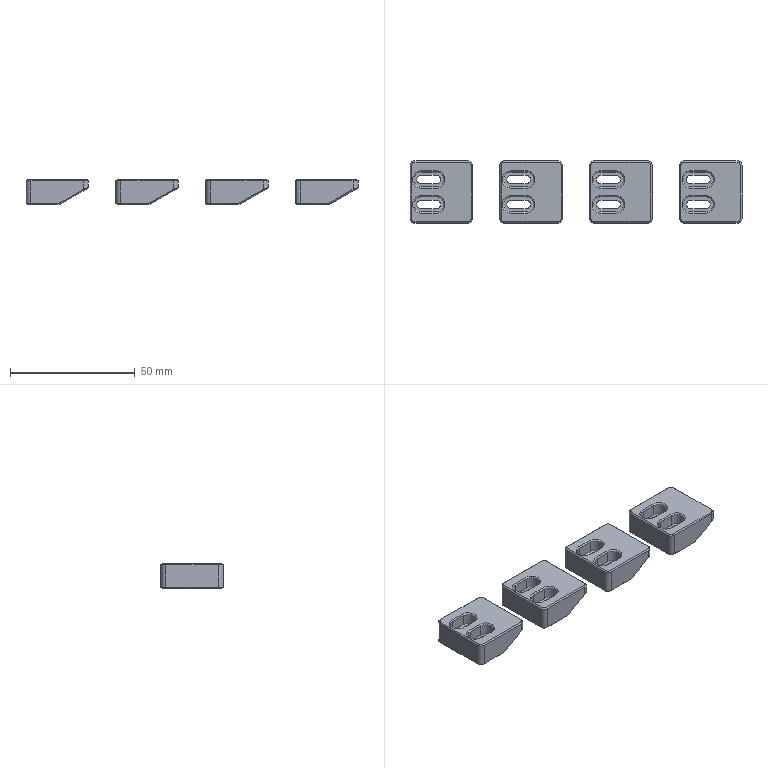NC program | NX | posted with a generic post | part box 133 x 25 x 10 mm
Lines 4147 to 5092 of 9691:
(ZLEVEL_PROFILE_1 , TOOL : D4R0.5)
N8274 T17 M6
N8276 G54
N8278 G17 G0 G90 X52.928 Y14.387 S9500 M3
N8280 G43 Z30. H17
N8282 Z1.492
N8284 G94 G1 Z-0.008 F1000.
N8286 X53.26 Y13.777
N8288 G3 X53.602 Y13.569 R0.4
N8290 G1 X54.449 Y13.548 F3500.
N8292 G2 X55.96 Y12.001 R1.548
N8294 G1 Y-12.002
N8296 G2 X54.447 Y-13.548 R1.546
N8298 G1 X53.731 Y-13.563
N8300 X53.733 Y-13.605 Z-0.012
N8302 Y-13.609 Z-0.017
N8304 X54.541 Y-13.585
N8306 G3 X56.077 Y-12.003 R1.583
N8308 G1 Y12.004
N8310 G3 X54.55 Y13.585 R1.583
N8312 G1 X53.602 Y13.618
N8314 Y13.651 Z-0.023
N8316 Y13.668 Z-0.03
N8318 G2 X54.868 Y13.578 R4.721
N8320 X56.185 Y12. R1.689
N8322 G1 Y-12.
N8324 G2 X54.868 Y-13.578 R1.689
N8326 X53.731 Y-13.668 R4.048
N8328 G1 Y-13.687 Z-0.037
N8330 Y-13.698 Z-0.045
N8332 G3 X54.868 Y-13.627 R4.522
N8334 X56.291 Y-12. R1.717
N8336 G1 Y12.
N8338 G3 X54.868 Y13.627 R1.717
N8340 X53.608 Y13.699 R5.373
N8342 G1 X53.616 Y13.731 Z-0.063
N8344 G2 X54.868 Y13.679 R7.793
N8346 X56.394 Y12. R1.79
N8348 G1 Y-12.
N8350 G2 X55.15 Y-13.595 R1.721
N8352 X53.731 Y-13.73 R4.1
N8354 G1 Y-13.759 Z-0.074
N8356 Y-13.768 Z-0.085
N8358 G3 X55.15 Y-13.649 R5.009
N8360 X56.495 Y-12. R1.779
N8362 G1 Y12.
N8364 G3 X55.077 Y13.665 R1.779
N8366 X53.626 Y13.768 R5.503
N8368 G1 X53.637 Y13.81 Z-0.108
N8370 G2 X55.15 Y13.693 R5.728
N8372 X56.594 Y12. R1.801
N8374 G1 Y-12.
N8376 G2 X55.431 Y-13.597 R1.737
N8378 X53.73 Y-13.81 R4.36
N8380 G1 X53.731 Y-13.827 Z-0.122
N8382 Y-13.84 Z-0.135
N8384 G3 X55.301 Y-13.696 R5.335
N8386 X56.693 Y-12. R1.829
N8388 G1 Y12.
N8390 G3 X55.301 Y13.696 R1.829
N8392 X53.731 Y13.84 R5.332
N8394 G1 X53.719 Y13.871 Z-0.164
N8396 G2 X55.311 Y13.739 R6.149
N8398 X56.79 Y12. R1.88
N8400 G1 Y-12.
N8402 G2 X55.311 Y-13.739 R1.88
N8404 X53.719 Y-13.871 R6.154
N8406 G1 X53.731 Y-13.904 Z-0.196
N8408 X54.565 Y-13.888
N8410 G3 X55.925 Y-13.542 R3.077
N8412 X56.886 Y-12. R1.785
N8414 G1 Y12.
N8416 G3 X55.431 Y13.747 R1.879
N8418 X53.731 Y13.904 R6.066
N8420 G1 X53.733 Y13.938 Z-0.231
N8422 G2 X55.431 Y13.785 R6.166
N8424 X56.835 Y12.686 R2.074
N8426 G1 X56.968 Y12.122
N8428 X56.981 Y12.
N8430 Y-12.
N8432 G2 X55.58 Y-13.743 R1.894
N8434 X53.733 Y-13.938 R5.951
N8436 G1 X53.724 Y-13.976 Z-0.269
N8438 X54.467 Y-13.962
N8440 G3 X55.991 Y-13.621 R3.913
N8442 X57.075 Y-12. R1.833
N8444 G1 Y12.002
N8446 G3 X56.499 Y13.277 R1.7
N8448 X55.431 Y13.824 R2.438
N8450 X53.724 Y13.976 R6.331
N8452 G1 X53.729 Y14.016 Z-0.309
N8454 G2 X55.994 Y13.678 R5.445
N8456 X57.168 Y12. R1.869
N8458 G1 Y-12.
N8460 G2 X55.994 Y-13.678 R1.869
N8462 X53.729 Y-14.016 R5.443
N8464 G1 X53.724 Y-14.058 Z-0.351
N8466 G3 X55.994 Y-13.721 R5.597
N8468 X57.259 Y-12. R1.893
N8470 G1 Y12.
N8472 G3 X55.994 Y13.721 R1.893
N8474 X53.724 Y14.058 R5.598
N8476 G1 X53.461 Y14.104 Z-0.397
N8478 X54.232 Y14.102
N8480 G2 X56.262 Y13.652 R4.836
N8482 X57.349 Y12. R1.88
N8484 G1 Y-12.
N8486 G2 X56.262 Y-13.652 R1.88
N8488 X54.232 Y-14.102 R4.837
N8490 G1 X53.461 Y-14.104
N8492 Y-14.151 Z-0.444
N8494 X54.2
N8496 G3 X56.513 Y-13.569 R4.883
N8498 G1 X56.557 Y-13.545
N8500 G3 X57.437 Y-12. R1.869
N8502 G1 Y12.005
N8504 G3 X56.504 Y13.572 R1.783
N8506 G1 X56.276 Y13.697
N8508 G3 X54.188 Y14.15 R5.072
N8510 G1 X53.461 Y14.151
N8512 Y14.2 Z-0.493
N8514 X54.196 Y14.199
N8516 G2 X56.554 Y13.598 R4.96
N8518 X57.522 Y12. R1.853
N8520 G1 Y-12.
N8522 G2 X56.517 Y-13.624 R1.88
N8524 X54.183 Y-14.2 R5.017
N8526 G1 X53.461
N8528 X53.742 Y-14.249 Z-0.542
N8530 G3 X56.557 Y-13.655 R5.49
N8532 X57.608 Y-12. R1.902
N8534 G1 Y12.
N8536 G3 X56.557 Y13.648 R1.875
N8538 X53.742 Y14.249 R5.381
N8540 G1 Y14.299 Z-0.592
N8542 G2 X56.808 Y13.557 R5.411
N8544 X57.694 Y12.005 R1.802
N8546 G1 Y-12.005
N8548 G2 X56.809 Y-13.557 R1.802
N8550 X53.742 Y-14.299 R5.409
N8552 G1 Y-14.324 Z-0.617
N8554 Y-14.349 Z-0.642
N8556 G3 X56.551 Y-13.749 R5.466
N8558 G1 X56.658 Y-13.695
N8560 G3 X57.78 Y-12. R1.933
N8562 G1 Y12.
N8564 G3 X56.658 Y13.695 R1.933
N8566 G1 X56.551 Y13.749
N8568 G3 X53.742 Y14.349 R5.467
N8570 G1 X53.747 Y14.374 Z-0.667
N8572 X53.751 Y14.399 Z-0.692
N8574 G2 X56.522 Y13.807 R5.412
N8576 G1 X56.745 Y13.695
N8578 G2 X57.867 Y12. R1.933
N8580 G1 Y-12.
N8582 G2 X56.745 Y-13.695 R1.933
N8584 G1 X56.522 Y-13.807
N8586 G2 X53.751 Y-14.399 R5.411
N8588 G1 X53.752 Y-14.424 Z-0.717
N8590 X53.753 Y-14.449 Z-0.742
N8592 G3 X56.493 Y-13.864 R5.353
N8594 G1 X56.832 Y-13.695
N8596 G3 X57.954 Y-12. R1.933
N8598 G1 Y12.
N8600 G3 X56.832 Y13.695 R1.933
N8602 G1 X56.493 Y13.864
N8604 G3 X53.753 Y14.449 R5.354
N8606 G1 X53.755 Y14.474 Z-0.767
N8608 X53.756 Y14.499 Z-0.792
N8610 G2 X56.465 Y13.922 R5.316
N8612 G1 X56.918 Y13.695
N8614 G2 X58.04 Y12. R1.933
N8616 G1 Y-12.
N8618 G2 X56.918 Y-13.695 R1.936
N8620 G1 X56.465 Y-13.922
N8622 G2 X53.756 Y-14.499 R5.315
N8624 G1 X53.758 Y-14.524 Z-0.817
N8626 X53.759 Y-14.549 Z-0.842
N8628 G3 X56.436 Y-13.98 R5.379
N8630 G1 X57.005 Y-13.695
N8632 G3 X58.127 Y-12. R1.933
N8634 G1 Y12.
N8636 G3 X57.005 Y13.695 R1.933
N8638 G1 X56.436 Y13.98
N8640 G3 X53.759 Y14.549 R5.266
N8642 G1 X53.76 Y14.574 Z-0.867
N8644 X53.762 Y14.599 Z-0.892
N8646 G2 X56.407 Y14.037 R5.221
N8648 G1 X57.091 Y13.695
N8650 G2 X58.214 Y12. R1.933
N8652 G1 Y-12.
N8654 G2 X57.091 Y-13.695 R1.933
N8656 G1 X56.407 Y-14.037
N8658 G2 X53.762 Y-14.599 R5.191
N8660 G1 X53.763 Y-14.624 Z-0.917
N8662 X53.764 Y-14.649 Z-0.942
N8664 G3 X56.378 Y-14.095 R5.178
N8666 G1 X57.178 Y-13.695
N8668 G3 X58.3 Y-12. R1.933
N8670 G1 Y12.
N8672 G3 X57.178 Y13.695 R1.933
N8674 G1 X56.378 Y14.095
N8676 G3 X53.764 Y14.649 R5.179
N8678 G1 X53.891 Y14.666 Z-0.959
N8680 X54.018 Y14.682 Z-0.976
N8682 X54.145 Y14.696 Z-0.992
N8684 G2 X56.349 Y14.153 R5.038
N8686 G1 X57.265 Y13.695
N8688 G2 X58.387 Y12. R1.933
N8690 G1 Y-12.
N8692 G2 X57.265 Y-13.695 R1.936
N8694 G1 X56.349 Y-14.153
N8696 G2 X54.135 Y-14.695 R5.021
N8698 G1 X54.275 Y-14.707 Z-1.005
N8700 X54.414 Y-14.711 Z-1.017
N8702 X54.553 Y-14.714 Z-1.03
N8704 X54.692 Y-14.71 Z-1.042
N8706 G3 X56.351 Y-14.195 R5.063
N8708 G1 X57.351 Y-13.695
N8710 G3 X58.473 Y-12. R1.933
N8712 G1 Y12.
N8714 G3 X57.351 Y13.695 R1.933
N8716 G1 X56.351 Y14.195
N8718 G3 X54.692 Y14.71 R5.042
N8720 G1 X54.825 Y14.714 Z-1.059
N8722 X54.957 Y14.705 Z-1.076
N8724 X55.087 Y14.694 Z-1.092
N8726 G2 X56.438 Y14.195 R5.676
N8728 G1 X57.438 Y13.695
N8730 G2 X58.56 Y12. R1.933
N8732 G1 Y-12.
N8734 G2 X57.438 Y-13.695 R1.933
N8736 G1 X56.438 Y-14.195
N8738 G2 X55.089 Y-14.694 R5.697
N8740 G1 X55.228 Y-14.691 Z-1.117
N8742 X55.363 Y-14.671 Z-1.142
N8744 G3 X56.353 Y-14.281 R6.036
N8746 G1 X57.524 Y-13.695
N8748 G3 X58.647 Y-12. R1.942
N8750 G1 Y12.
N8752 G3 X57.524 Y13.695 R1.933
N8754 G1 X56.355 Y14.28
N8756 G3 X55.361 Y14.671 R6.026
N8758 G1 X55.476 Y14.662 Z-1.167
N8760 X55.59 Y14.648 Z-1.192
N8762 G2 X56.405 Y14.298 R7.558
N8764 G1 X57.611 Y13.695
N8766 G2 X58.733 Y12. R1.933
N8768 G1 Y-12.
N8770 G2 X57.611 Y-13.695 R1.933
N8772 G1 X56.396 Y-14.303
N8774 G2 X55.593 Y-14.647 R7.478
N8776 G1 X55.688 Y-14.64 Z-1.217
N8778 X55.779 Y-14.624 Z-1.242
N8780 G3 X56.473 Y-14.308 R10.854
N8782 G1 X57.698 Y-13.695
N8784 G3 X58.82 Y-12. R1.933
N8786 G1 Y12.
N8788 G3 X57.698 Y13.695 R1.933
N8790 G1 X56.698 Y14.195
N8792 G3 X55.777 Y14.625 R16.455
N8794 G1 X55.852 Y14.617 Z-1.267
N8796 X55.926 Y14.606 Z-1.292
N8798 X56.784 Y14.195
N8800 X57.784 Y13.695
N8802 G2 X58.906 Y12. R1.933
N8804 G1 Y-12.
N8806 G2 X57.784 Y-13.695 R1.942
N8808 G1 X56.784 Y-14.195
N8810 X55.929 Y-14.606
N8812 X56.057 Y-14.593 Z-1.342
N8814 X56.871 Y-14.195
N8816 X57.871 Y-13.695
N8818 G3 X58.993 Y-12. R1.933
N8820 G1 Y12.
N8822 G3 X57.871 Y13.695 R1.933
N8824 G1 X56.871 Y14.195
N8826 X56.055 Y14.592
N8828 X56.168 Y14.582 Z-1.392
N8830 X56.276 Y14.533
N8832 X56.957 Y14.195
N8834 X57.957 Y13.695
N8836 G2 X59.08 Y12. R1.933
N8838 G1 Y-12.
N8840 G2 X57.957 Y-13.695 R1.933
N8842 G1 X56.957 Y-14.195
N8844 X56.276 Y-14.534
N8846 X56.17 Y-14.583
N8848 X56.281 Y-14.575 Z-1.442
N8850 X57.044 Y-14.195
N8852 X58.044 Y-13.695
N8854 G3 X59.166 Y-12. R1.936
N8856 G1 Y12.
N8858 G3 X58.044 Y13.695 R1.933
N8860 G1 X57.044 Y14.195
N8862 X56.279 Y14.574
N8864 X56.367 Y14.571 Z-1.492
N8866 X57.131 Y14.195
N8868 X58.131 Y13.695
N8870 G2 X59.253 Y12. R1.933
N8872 G1 Y-12.
N8874 G2 X58.131 Y-13.695 R1.933
N8876 G1 X57.131 Y-14.195
N8878 X56.369 Y-14.571
N8880 X56.457 Z-1.542
N8882 X56.557 Y-14.524
N8884 X57.217 Y-14.195
N8886 X58.217 Y-13.695
N8888 G3 X59.339 Y-12. R1.933
N8890 G1 Y12.
N8892 G3 X58.217 Y13.695 R1.933
N8894 G1 X57.217 Y14.195
N8896 X56.557 Y14.523
N8898 X56.455 Y14.57
N8900 X56.545 Y14.571 Z-1.592
N8902 X57.304 Y14.195
N8904 X58.304 Y13.695
N8906 G2 X59.426 Y12. R1.933
N8908 G1 Y-12.
N8910 G2 X58.304 Y-13.695 R1.933
N8912 G1 X57.304 Y-14.195
N8914 X56.547 Y-14.572
N8916 X56.634 Y-14.569 Z-1.642
N8918 X57.39 Y-14.195
N8920 X58.39 Y-13.695
N8922 G3 X59.513 Y-12. R1.936
N8924 G1 Y12.
N8926 G3 X58.39 Y13.695 R1.933
N8928 G1 X57.39 Y14.195
N8930 X56.633 Y14.569
N8932 X56.721 Y14.567 Z-1.692
N8934 X56.838 Y14.512
N8936 X57.477 Y14.195
N8938 X58.477 Y13.695
N8940 G2 X59.599 Y12. R1.933
N8942 G1 Y-12.
N8944 G2 X58.477 Y-13.695 R1.933
N8946 G1 X57.477 Y-14.195
N8948 X56.838 Y-14.513
N8950 X56.722 Y-14.568
N8952 X56.812 Y-14.569 Z-1.742
N8954 X56.838 Y-14.557
N8956 X57.564 Y-14.195
N8958 X58.564 Y-13.695
N8960 G3 X59.686 Y-12. R1.933
N8962 G1 Y12.
N8964 G3 X58.564 Y13.695 R1.933
N8966 G1 X57.564 Y14.195
N8968 X56.838 Y14.556
N8970 X56.81 Y14.568
N8972 X56.898 Y14.567 Z-1.792
N8974 X57.65 Y14.195
N8976 X58.65 Y13.695
N8978 G2 X59.772 Y12. R1.933
N8980 G1 Y-12.
N8982 G2 X58.65 Y-13.695 R1.942
N8984 G1 X57.65 Y-14.195
N8986 X56.899 Y-14.567
N8988 X56.987 Y-14.565 Z-1.842
N8990 X57.12 Y-14.503
N8992 X57.737 Y-14.195
N8994 X58.737 Y-13.695
N8996 G3 X59.859 Y-12. R1.933
N8998 G1 Y12.
N9000 G3 X58.737 Y13.695 R1.933
N9002 G1 X57.737 Y14.195
N9004 X57.12 Y14.502
N9006 X56.986 Y14.565
N9008 X57.075 Y14.566 Z-1.892
N9010 X57.12 Y14.546
N9012 X57.823 Y14.195
N9014 X58.824 Y13.695
N9016 G2 X59.946 Y12. R1.933
N9018 G1 Y-12.
N9020 G2 X58.824 Y-13.695 R1.933
N9022 G1 X57.823 Y-14.195
N9024 X57.12 Y-14.546
N9026 X57.077 Y-14.566
N9028 X57.165 Y-14.565 Z-1.942
N9030 X57.91 Y-14.195
N9032 X58.91 Y-13.695
N9034 G3 X60.032 Y-12. R1.942
N9036 G1 Y12.
N9038 G3 X58.91 Y13.695 R1.933
N9040 G1 X57.91 Y14.195
N9042 X57.164 Y14.565
N9044 X57.252 Y14.563 Z-1.992
N9046 X57.401 Y14.492
N9048 X57.997 Y14.195
N9050 X58.997 Y13.695
N9052 G2 X60.119 Y12. R1.933
N9054 G1 Y-12.
N9056 G2 X58.997 Y-13.695 R1.933
N9058 G1 X57.997 Y-14.195
N9060 X57.401 Y-14.493
N9062 X57.253 Y-14.563
N9064 X57.342 Z-2.042
N9066 X57.401 Y-14.536
N9068 X58.083 Y-14.195
N9070 X59.083 Y-13.695
N9072 G3 X60.205 Y-12. R1.933
N9074 G1 Y12.
N9076 G3 X59.083 Y13.695 R1.933
N9078 G1 X58.083 Y14.195
N9080 X57.401 Y14.535
N9082 X57.341 Y14.563
N9084 X57.43 Z-2.092
N9086 X58.17 Y14.195
N9088 X59.17 Y13.695
N9090 G2 X60.292 Y12. R1.933
N9092 G1 Y-12.
N9094 G2 X59.17 Y-13.695 R1.936
N9096 G1 X58.17 Y-14.195
N9098 X57.43 Y-14.563
N9100 X57.518 Y-14.561 Z-2.142
N9102 X58.256 Y-14.195
N9104 X59.257 Y-13.695
N9106 G3 X60.379 Y-12. R1.933
N9108 G1 Y12.
N9110 G3 X59.257 Y13.695 R1.933
N9112 G1 X58.256 Y14.195
N9114 X57.517 Y14.561
N9116 X57.606 Y14.56 Z-2.192
N9118 X57.683 Y14.525
N9120 X58.343 Y14.195
N9122 X59.343 Y13.695
N9124 G2 X60.465 Y12. R1.933
N9126 G1 Y-12.
N9128 G2 X59.343 Y-13.695 R1.933
N9130 G1 X58.343 Y-14.195
N9132 X57.683 Y-14.526
N9134 X57.607 Y-14.561
N9136 X57.696 Y-14.562 Z-2.242
N9138 X58.43 Y-14.195
N9140 X59.43 Y-13.695
N9142 G3 X60.552 Y-12. R1.933
N9144 G1 Y12.
N9146 G3 X59.43 Y13.695 R1.933
N9148 G1 X58.43 Y14.195
N9150 X57.695 Y14.562
N9152 X57.782 Y14.559 Z-2.292
N9154 X58.516 Y14.195
N9156 X59.516 Y13.695
N9158 G2 X60.638 Y12. R1.933
N9160 G1 Y-12.
N9162 G2 X59.516 Y-13.695 R1.936
N9164 G1 X58.516 Y-14.195
N9166 X57.782 Y-14.559
N9168 X57.87 Y-14.558 Z-2.342
N9170 X57.964 Y-14.515
N9172 X58.603 Y-14.195
N9174 X59.603 Y-13.695
N9176 G3 X60.725 Y-12. R1.933
N9178 G1 Y12.
N9180 G3 X59.603 Y13.695 R1.933
N9182 G1 X58.603 Y14.195
N9184 X57.964 Y14.514
N9186 X57.869 Y14.558
N9188 X57.958 Y14.56 Z-2.392
N9190 X58.689 Y14.195
N9192 X59.69 Y13.695
N9194 G2 X60.812 Y12. R1.933
N9196 G1 Y-12.
N9198 G2 X59.69 Y-13.695 R1.933
N9200 G1 X58.689 Y-14.195
N9202 X57.959 Y-14.561
N9204 X58.045 Y-14.558 Z-2.442
N9206 X58.776 Y-14.195
N9208 X59.776 Y-13.695
N9210 G3 X60.898 Y-12. R1.942
N9212 G1 Y12.
N9214 G3 X59.776 Y13.695 R1.933
N9216 G1 X58.776 Y14.195
N9218 X58.045 Y14.557
N9220 X58.132 Y14.556 Z-2.492
N9222 X58.246 Y14.504
N9224 X58.863 Y14.195
N9226 X59.863 Y13.695
N9228 G2 X60.985 Y12. R1.933
N9230 G1 Y-12.
N9232 G2 X59.863 Y-13.695 R1.933
N9234 G1 X58.863 Y-14.195
N9236 X58.246 Y-14.504
N9238 X58.133 Y-14.557
N9240 X58.221 Y-14.558 Z-2.542
N9242 X58.246 Y-14.547
N9244 X58.949 Y-14.195
N9246 X59.949 Y-13.695
N9248 G3 X61.071 Y-12. R1.933
N9250 G1 Y12.
N9252 G3 X59.949 Y13.695 R1.933
N9254 G1 X58.949 Y14.195
N9256 X58.246 Y14.547
N9258 X58.221 Y14.558
N9260 X58.308 Y14.556 Z-2.592
N9262 X59.036 Y14.195
N9264 X60.036 Y13.695
N9266 G2 X61.158 Y12. R1.933
N9268 G1 Y-12.
N9270 G2 X60.036 Y-13.695 R1.942
N9272 G1 X59.036 Y-14.195
N9274 X58.308 Y-14.556
N9276 X58.395 Y-14.555 Z-2.642
N9278 X58.527 Y-14.493
N9280 X59.122 Y-14.195
N9282 X60.123 Y-13.695
N9284 G3 X61.245 Y-12. R1.933
N9286 G1 Y12.
N9288 G3 X60.123 Y13.695 R1.933
N9290 G1 X59.122 Y14.195
N9292 X58.527 Y14.493
N9294 X58.395 Y14.555
N9296 X58.483 Y14.556 Z-2.692
N9298 X58.527 Y14.536
N9300 X59.209 Y14.195
N9302 X60.209 Y13.695
N9304 G2 X61.331 Y12. R1.933
N9306 G1 Y-12.
N9308 G2 X60.209 Y-13.695 R1.933
N9310 G1 X59.209 Y-14.195
N9312 X58.527 Y-14.536
N9314 X58.484 Y-14.556
N9316 X58.571 Y-14.555 Z-2.742
N9318 X59.296 Y-14.195
N9320 X60.296 Y-13.695
N9322 G3 X61.418 Y-12. R1.936
N9324 G1 Y12.
N9326 G3 X60.296 Y13.695 R1.933
N9328 G1 X59.296 Y14.195
N9330 X58.571 Y14.555
N9332 X58.658 Y14.553 Z-2.792
N9334 X59.382 Y14.195
N9336 X60.382 Y13.695
N9338 G2 X61.504 Y12. R1.933
N9340 G1 Y-12.
N9342 G2 X60.382 Y-13.695 R1.933
N9344 G1 X59.382 Y-14.195
N9346 X58.658 Y-14.553
N9348 X58.746 Y-14.554 Z-2.842
N9350 X58.809 Y-14.526
N9352 X59.469 Y-14.195
N9354 X60.469 Y-13.695
N9356 G3 X61.591 Y-12. R1.933
N9358 G1 Y12.
N9360 G3 X60.469 Y13.695 R1.933
N9362 G1 X59.469 Y14.195
N9364 X58.809 Y14.525
N9366 X58.746 Y14.554
N9368 X58.834 Z-2.892
N9370 X59.556 Y14.195
N9372 X60.556 Y13.695
N9374 G2 X61.678 Y12. R1.933
N9376 G1 Y-12.
N9378 G2 X60.556 Y-13.695 R1.933
N9380 G1 X59.556 Y-14.195
N9382 X58.835 Y-14.555
N9384 X58.921 Y-14.552 Z-2.942
N9386 X59.642 Y-14.195
N9388 X60.642 Y-13.695
N9390 G3 X61.764 Y-12. R1.936
N9392 G1 Y12.
N9394 G3 X60.642 Y13.695 R1.933
N9396 G1 X59.642 Y14.195
N9398 X58.921 Y14.552
N9400 X59.009 Z-2.992
N9402 X59.09 Y14.514
N9404 X59.729 Y14.195
N9406 X60.729 Y13.695
N9408 G2 X61.851 Y12. R1.933
N9410 G1 Y-12.
N9412 G2 X60.729 Y-13.695 R1.933
N9414 G1 X59.729 Y-14.195
N9416 X59.09 Y-14.515
N9418 X59.009 Y-14.552
N9420 X59.098 Y-14.554 Z-3.042
N9422 X59.815 Y-14.195
N9424 X60.815 Y-13.695
N9426 G3 X61.937 Y-12. R1.933
N9428 G1 Y12.
N9430 G3 X60.815 Y13.695 R1.933
N9432 G1 X59.815 Y14.195
N9434 X59.097 Y14.554
N9436 X59.183 Y14.551 Z-3.092
N9438 X59.902 Y14.195
N9440 X60.902 Y13.695
N9442 G2 X62.024 Y12. R1.933
N9444 G1 Y-12.
N9446 G2 X60.902 Y-13.695 R1.942
N9448 G1 X59.902 Y-14.195
N9450 X59.184 Y-14.551
N9452 X59.271 Y-14.55 Z-3.142
N9454 X59.372 Y-14.504
N9456 X59.989 Y-14.195
N9458 X60.989 Y-13.695
N9460 G3 X62.111 Y-12. R1.933
N9462 G1 Y12.
N9464 G3 X60.989 Y13.695 R1.933
N9466 G1 X59.989 Y14.195
N9468 X59.372 Y14.504
N9470 X59.271 Y14.55
N9472 X59.359 Y14.552 Z-3.192
N9474 X60.075 Y14.195
N9476 X61.075 Y13.695
N9478 G2 X62.197 Y12. R1.933
N9480 G1 Y-12.
N9482 G2 X61.075 Y-13.695 R1.933
N9484 G1 X60.075 Y-14.195
N9486 X59.36 Y-14.553
N9488 X59.446 Y-14.55 Z-3.242
N9490 X60.162 Y-14.195
N9492 X61.162 Y-13.695
N9494 G3 X62.284 Y-12. R1.942
N9496 G1 Y12.
N9498 G3 X61.162 Y13.695 R1.933
N9500 G1 X60.162 Y14.195
N9502 X59.445 Y14.55
N9504 X59.532 Y14.549 Z-3.292
N9506 X59.653 Y14.493
N9508 X60.248 Y14.195
N9510 X61.248 Y13.695
N9512 G2 X62.37 Y12. R1.933
N9514 G1 Y-12.
N9516 G2 X61.248 Y-13.695 R1.933
N9518 G1 X60.248 Y-14.195
N9520 X59.653 Y-14.493
N9522 X59.533 Y-14.549
N9524 X59.621 Y-14.551 Z-3.342
N9526 X59.653 Y-14.536
N9528 X60.335 Y-14.195
N9530 X61.335 Y-13.695
N9532 G3 X62.457 Y-12. R1.933
N9534 G1 Y12.
N9536 G3 X61.335 Y13.695 R1.933
N9538 G1 X60.335 Y14.195
N9540 X59.653 Y14.536
N9542 X59.62 Y14.551
N9544 X59.707 Y14.55 Z-3.392
N9546 X60.422 Y14.195
N9548 X61.422 Y13.695
N9550 G2 X62.544 Y12. R1.933
N9552 G1 Y-12.
N9554 G2 X61.422 Y-13.695 R1.936
N9556 G1 X60.422 Y-14.195
N9558 X59.707 Y-14.55
N9560 X59.794 Y-14.548 Z-3.442
N9562 X59.935 Y-14.482
N9564 X60.508 Y-14.195
N9566 X61.508 Y-13.695
N9568 G3 X62.63 Y-12. R1.933
N9570 G1 Y12.
N9572 G3 X61.508 Y13.695 R1.933
N9574 G1 X60.508 Y14.195
N9576 X59.935 Y14.482
N9578 X59.793 Y14.548
N9580 X59.881 Y14.549 Z-3.492
N9582 X59.935 Y14.525
N9584 X60.595 Y14.195
N9586 X61.595 Y13.695
N9588 G2 X62.717 Y12. R1.933
N9590 G1 Y-12.
N9592 G2 X61.595 Y-13.695 R1.933
N9594 G1 X60.595 Y-14.195
N9596 X59.935 Y-14.526
N9598 X59.882 Y-14.549
N9600 X59.969 Z-3.542
N9602 X60.681 Y-14.195
N9604 X61.681 Y-13.695
N9606 G3 X62.803 Y-12. R1.933
N9608 G1 Y12.
N9610 G3 X61.681 Y13.695 R1.933
N9612 G1 X60.681 Y14.195
N9614 X59.969 Y14.55
N9616 X60.055 Y14.547 Z-3.592
N9618 X60.768 Y14.195
N9620 X61.768 Y13.695
N9622 G2 X62.89 Y12. R1.933
N9624 G1 Y-12.
N9626 G2 X61.768 Y-13.695 R1.936
N9628 G1 X60.768 Y-14.195
N9630 X60.056 Y-14.547
N9632 X60.143 Y-14.548 Z-3.642
N9634 X60.216 Y-14.515
N9636 X60.855 Y-14.195
N9638 X61.855 Y-13.695
N9640 G3 X62.977 Y-12. R1.933
N9642 G1 Y12.
N9644 G3 X61.855 Y13.695 R1.933
N9646 G1 X60.855 Y14.195
N9648 X60.216 Y14.514
N9650 X60.143 Y14.548
N9652 X60.231 Y14.549 Z-3.692
N9654 X60.941 Y14.195
N9656 X61.941 Y13.695
N9658 G2 X63.063 Y12. R1.933
N9660 G1 Y-12.
N9662 G2 X61.941 Y-13.695 R1.933
N9664 G1 X60.941 Y-14.195
N9666 X60.231 Y-14.549
N9668 X60.317 Y-14.546 Z-3.742
N9670 X61.028 Y-14.195
N9672 X62.028 Y-13.695
N9674 G3 X63.15 Y-12. R1.942
N9676 G1 Y12.
N9678 G3 X62.028 Y13.695 R1.933
N9680 G1 X61.028 Y14.195
N9682 X60.317 Y14.546
N9684 X60.404 Z-3.792
N9686 X60.497 Y14.504
N9688 X61.114 Y14.195
N9690 X62.114 Y13.695
N9692 G2 X63.236 Y12. R1.933
N9694 G1 Y-12.
N9696 G2 X62.114 Y-13.695 R1.933
N9698 G1 X61.114 Y-14.195
N9700 X60.497 Y-14.504
N9702 X60.405 Y-14.546
N9704 X60.493 Y-14.549 Z-3.842
N9706 X61.201 Y-14.195
N9708 X62.201 Y-13.695
N9710 G3 X63.323 Y-12. R1.933
N9712 G1 Y12.
N9714 G3 X62.201 Y13.695 R1.933
N9716 G1 X61.201 Y14.195
N9718 X60.492 Y14.549
N9720 X60.578 Y14.546 Z-3.892
N9722 X61.288 Y14.195
N9724 X62.288 Y13.695
N9726 G2 X63.41 Y12. R1.933
N9728 G1 Y-12.
N9730 G2 X62.288 Y-13.695 R1.942
N9732 G1 X61.288 Y-14.195
N9734 X60.579 Y-14.546
N9736 X60.666 Y-14.545 Z-3.942
N9738 X60.779 Y-14.493
N9740 X61.374 Y-14.195
N9742 X62.374 Y-13.695
N9744 G3 X63.496 Y-12. R1.933
N9746 G1 Y12.
N9748 G3 X62.374 Y13.695 R1.933
N9750 G1 X61.374 Y14.195
N9752 X60.779 Y14.493
N9754 X60.665 Y14.545
N9756 X60.753 Y14.547 Z-3.992
N9758 X60.779 Y14.536
N9760 X61.461 Y14.195
N9762 X62.461 Y13.695
N9764 G2 X63.583 Y12. R1.933
N9766 G1 Y-12.
N9768 G2 X62.461 Y-13.695 R1.933
N9770 G1 X61.461 Y-14.195
N9772 X60.779 Y-14.536
N9774 X60.754 Y-14.547
N9776 X60.841 Y-14.545 Z-4.042
N9778 X61.547 Y-14.195
N9780 X62.547 Y-13.695
N9782 G3 X63.669 Y-12. R1.936
N9784 G1 Y12.
N9786 G3 X62.547 Y13.695 R1.933
N9788 G1 X61.547 Y14.195
N9790 X60.84 Y14.546
N9792 X60.927 Y14.544 Z-4.092
N9794 X61.06 Y14.482
N9796 X61.634 Y14.195
N9798 X62.634 Y13.695
N9800 G2 X63.756 Y12. R1.933
N9802 G1 Y-12.
N9804 G2 X62.634 Y-13.695 R1.933
N9806 G1 X61.634 Y-14.195
N9808 X61.06 Y-14.482
N9810 X60.928 Y-14.544
N9812 X61.016 Y-14.545 Z-4.142
N9814 X61.06 Y-14.526
N9816 X61.721 Y-14.195
N9818 X62.721 Y-13.695
N9820 G3 X63.843 Y-12. R1.933
N9822 G1 Y12.
N9824 G3 X62.721 Y13.695 R1.933
N9826 G1 X61.721 Y14.195
N9828 X61.06 Y14.525
N9830 X61.015 Y14.546
N9832 X61.102 Y14.545 Z-4.192
N9834 X61.807 Y14.195
N9836 X62.807 Y13.695
N9838 G2 X63.929 Y12. R1.933
N9840 G1 Y-12.
N9842 G2 X62.807 Y-13.695 R1.933
N9844 G1 X61.807 Y-14.195
N9846 X61.103 Y-14.545
N9848 X61.189 Y-14.543 Z-4.242
N9850 X61.894 Y-14.195
N9852 X62.894 Y-13.695
N9854 G3 X64.016 Y-12. R1.936
N9856 G1 Y12.
N9858 G3 X62.894 Y13.695 R1.933
N9860 G1 X61.894 Y14.195
N9862 X61.188 Y14.543
N9864 X61.276 Y14.544 Z-4.292
N9866 X61.342 Y14.514
N9868 X61.98 Y14.195
N9870 X62.98 Y13.695
N9872 G2 X64.102 Y12. R1.933
N9874 G1 Y-12.
N9876 G2 X62.98 Y-13.695 R1.933
N9878 G1 X61.98 Y-14.195
N9880 X61.342 Y-14.515
N9882 X61.277 Y-14.544
N9884 X61.365 Y-14.545 Z-4.342
N9886 X62.067 Y-14.195
N9888 X63.067 Y-13.695
N9890 G3 X64.189 Y-12. R1.933
N9892 G1 Y12.
N9894 G3 X63.067 Y13.695 R1.933
N9896 G1 X62.067 Y14.195
N9898 X61.364 Y14.545
N9900 X61.45 Y14.543 Z-4.392
N9902 X62.154 Y14.195
N9904 X63.154 Y13.695
N9906 G2 X64.276 Y12. R1.933
N9908 G1 Y-12.
N9910 G2 X63.154 Y-13.695 R1.942
N9912 G1 X62.154 Y-14.195
N9914 X61.451 Y-14.542
N9916 X61.538 Z-4.442
N9918 X61.623 Y-14.504
N9920 X62.24 Y-14.195
N9922 X63.24 Y-13.695
N9924 G3 X64.362 Y-12. R1.933
N9926 G1 Y12.
N9928 G3 X63.24 Y13.695 R1.933
N9930 G1 X62.24 Y14.195
N9932 X61.623 Y14.504
N9934 X61.537 Y14.543
N9936 X61.626 Y14.546 Z-4.492
N9938 X62.327 Y14.195
N9940 X63.327 Y13.695
N9942 G2 X64.449 Y12. R1.933
N9944 G1 Y-12.
N9946 G2 X63.327 Y-13.695 R1.933
N9948 G1 X62.327 Y-14.195
N9950 X61.627 Y-14.545
N9952 X61.713 Y-14.542 Z-4.542
N9954 X62.413 Y-14.195
N9956 X63.413 Y-13.695
N9958 G3 X64.535 Y-12. R1.942
N9960 G1 Y12.
N9962 G3 X63.413 Y13.695 R1.933
N9964 G1 X62.413 Y14.195
N9966 X61.711 Y14.542
N9968 X61.799 Y14.541 Z-4.592
N9970 X61.905 Y14.493
N9972 X62.5 Y14.195
N9974 X63.5 Y13.695
N9976 G2 X64.622 Y12. R1.933
N9978 G1 Y-12.
N9980 G2 X63.5 Y-13.695 R1.933
N9982 G1 X62.5 Y-14.195
N9984 X61.905 Y-14.493
N9986 X61.8 Y-14.541
N9988 X61.889 Y-14.543 Z-4.642
N9990 X62.587 Y-14.195
N9992 X63.587 Y-13.695
N9994 G3 X64.709 Y-12. R1.933
N9996 G1 Y12.
N9998 G3 X63.587 Y13.695 R1.933
N10000 G1 X62.587 Y14.195
N10002 X61.887 Y14.544
N10004 X61.973 Y14.542 Z-4.692
N10006 X62.673 Y14.195
N10008 X63.673 Y13.695
N10010 G2 X64.795 Y12. R1.933
N10012 G1 Y-12.
N10014 G2 X63.673 Y-13.695 R1.936
N10016 G1 X62.673 Y-14.195
N10018 X61.975 Y-14.541
N10020 X62.061 Y-14.54 Z-4.742
N10022 X62.186 Y-14.482
N10024 X62.76 Y-14.195
N10026 X63.76 Y-13.695
N10028 G3 X64.882 Y-12. R1.933
N10030 G1 Y12.
N10032 G3 X63.76 Y13.695 R1.933
N10034 G1 X62.76 Y14.195
N10036 X62.186 Y14.482
N10038 X62.06 Y14.54
N10040 X62.148 Y14.542 Z-4.792
N10042 X62.186 Y14.525
N10044 X62.846 Y14.195
N10046 X63.846 Y13.695
N10048 G2 X64.969 Y12. R1.933
N10050 G1 Y-12.
N10052 G2 X63.846 Y-13.695 R1.933
N10054 G1 X62.846 Y-14.195
N10056 X62.186 Y-14.526
N10058 X62.15 Y-14.542
N10060 X62.237 Y-14.541 Z-4.842
N10062 X62.933 Y-14.195
N10064 X63.933 Y-13.695
N10066 G3 X65.055 Y-12. R1.933
N10068 G1 Y12.
N10070 G3 X63.933 Y13.695 R1.933
N10072 G1 X62.933 Y14.195
N10074 X62.235 Y14.541
N10076 X62.322 Y14.539 Z-4.892
N10078 X63.02 Y14.195
N10080 X64.02 Y13.695
N10082 G2 X65.142 Y12. R1.933
N10084 G1 Y-12.
N10086 G2 X64.02 Y-13.695 R1.936
N10088 G1 X63.02 Y-14.195
N10090 X62.324 Y-14.539
N10092 X62.412 Y-14.54 Z-4.942
N10094 X62.468 Y-14.515
N10096 X63.106 Y-14.195
N10098 X64.106 Y-13.695
N10100 G3 X65.228 Y-12. R1.933
N10102 G1 Y12.
N10104 G3 X64.106 Y13.695 R1.933
N10106 G1 X62.468 Y14.514
N10108 X62.41 Y14.54
N10110 X62.498 Y14.541 Z-4.992
N10112 X63.193 Y14.195
N10114 X64.193 Y13.695
N10116 G2 X65.315 Y12. R1.933
N10118 G1 Y-12.
N10120 G2 X64.193 Y-13.695 R1.933
N10122 G1 X63.193 Y-14.195
N10124 X62.5 Y-14.54
N10126 X62.586 Y-14.537 Z-5.042
N10128 X63.279 Y-14.195
N10130 X64.279 Y-13.695
N10132 G3 X65.402 Y-12. R1.942
N10134 G1 Y12.
N10136 G3 X64.279 Y13.695 R1.933
N10138 G1 X63.279 Y14.195
N10140 X62.585 Y14.538
N10142 X62.673 Z-5.092
N10144 X62.749 Y14.504
N10146 X63.366 Y14.195
N10148 X64.366 Y13.695
N10150 G2 X65.488 Y12. R1.933
N10152 G1 Y-12.
N10154 G2 X64.366 Y-13.695 R1.933
N10156 G1 X63.366 Y-14.195
N10158 X62.749 Y-14.504